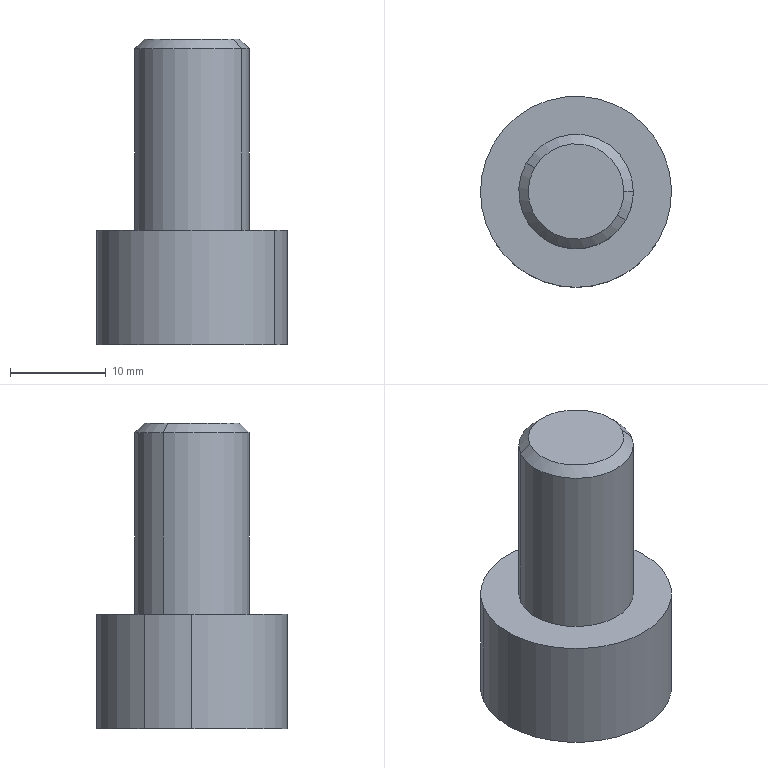Part | SolidWorks | features BaseBody 1 | 1 solid | 19 faces | box 20 x 20 x 32 mm | volume 5504 mm3 | plane 10 | cylinder 6 | cone 3 | commonest cylinder face diameters 12 x3 20 x3
STEP:
#1=CARTESIAN_POINT('',(364.67,895.749,656.107));
#2=VERTEX_POINT('',#1);
#3=CARTESIAN_POINT('',(363.804,896.249,655.107));
#4=VERTEX_POINT('',#3);
#5=CARTESIAN_POINT('',(364.67,895.749,656.107));
#6=DIRECTION('',(-0.6124,0.3536,-0.7071));
#7=VECTOR('',#6,1000.);
#8=LINE('',#5,#7);
#9=EDGE_CURVE('',#2,#4,#8,.T.);
#10=ORIENTED_EDGE('',*,*,#9,.T.);
#11=CARTESIAN_POINT('',(374.196,890.249,655.107));
#12=VERTEX_POINT('',#11);
#13=CARTESIAN_POINT('',(369.,893.249,655.107));
#14=DIRECTION('',(0.,0.,1.));
#15=DIRECTION('',(-0.866,0.5,0.));
#16=AXIS2_PLACEMENT_3D('',#13,#14,#15);
#17=CIRCLE('',#16,6.);
#18=EDGE_CURVE('',#4,#12,#17,.T.);
#19=ORIENTED_EDGE('',*,*,#18,.T.);
#20=CARTESIAN_POINT('',(373.33,890.749,656.107));
#21=VERTEX_POINT('',#20);
#22=CARTESIAN_POINT('',(373.33,890.749,656.107));
#23=DIRECTION('',(0.6124,-0.3536,-0.7071));
#24=VECTOR('',#23,1000.);
#25=LINE('',#22,#24);
#26=EDGE_CURVE('',#21,#12,#25,.T.);
#27=ORIENTED_EDGE('',*,*,#26,.F.);
#28=CARTESIAN_POINT('',(369.,893.249,656.107));
#29=DIRECTION('',(0.,0.,-1.));
#30=DIRECTION('',(-0.866,0.5,0.));
#31=AXIS2_PLACEMENT_3D('',#28,#29,#30);
#32=CIRCLE('',#31,5.);
#33=EDGE_CURVE('',#21,#2,#32,.T.);
#34=ORIENTED_EDGE('',*,*,#33,.T.);
#35=EDGE_LOOP('',(#10,#19,#27,#34));
#36=FACE_OUTER_BOUND('',#35,.T.);
#37=CARTESIAN_POINT('',(369.,893.249,656.107));
#38=DIRECTION('',(0.,0.,-1.));
#39=DIRECTION('',(1.,0.,0.));
#40=AXIS2_PLACEMENT_3D('',#37,#38,#39);
#41=CONICAL_SURFACE('',#40,5.,0.7854);
#42=ADVANCED_FACE('',(#36),#41,.T.);
#43=ORIENTED_EDGE('',*,*,#33,.F.);
#44=CARTESIAN_POINT('',(374.,893.249,656.107));
#45=VERTEX_POINT('',#44);
#46=CARTESIAN_POINT('',(369.,893.249,656.107));
#47=DIRECTION('',(0.,0.,-1.));
#48=DIRECTION('',(-0.866,0.5,0.));
#49=AXIS2_PLACEMENT_3D('',#46,#47,#48);
#50=CIRCLE('',#49,5.);
#51=EDGE_CURVE('',#45,#21,#50,.T.);
#52=ORIENTED_EDGE('',*,*,#51,.F.);
#53=CARTESIAN_POINT('',(369.,893.249,656.107));
#54=DIRECTION('',(0.,0.,-1.));
#55=DIRECTION('',(-0.866,0.5,0.));
#56=AXIS2_PLACEMENT_3D('',#53,#54,#55);
#57=CIRCLE('',#56,5.);
#58=EDGE_CURVE('',#2,#45,#57,.T.);
#59=ORIENTED_EDGE('',*,*,#58,.F.);
#60=EDGE_LOOP('',(#43,#52,#59));
#61=FACE_OUTER_BOUND('',#60,.T.);
#62=CARTESIAN_POINT('',(369.,893.249,656.107));
#63=DIRECTION('',(0.,0.,1.));
#64=DIRECTION('',(1.,0.,0.));
#65=AXIS2_PLACEMENT_3D('',#62,#63,#64);
#66=PLANE('',#65);
#67=ADVANCED_FACE('',(#61),#66,.T.);
#68=CARTESIAN_POINT('',(363.804,896.249,636.107));
#69=VERTEX_POINT('',#68);
#70=CARTESIAN_POINT('',(363.804,896.249,656.107));
#71=DIRECTION('',(0.,0.,-1.));
#72=VECTOR('',#71,1000.);
#73=LINE('',#70,#72);
#74=EDGE_CURVE('',#4,#69,#73,.T.);
#75=ORIENTED_EDGE('',*,*,#74,.T.);
#76=CARTESIAN_POINT('',(374.196,890.249,636.107));
#77=VERTEX_POINT('',#76);
#78=CARTESIAN_POINT('',(369.,893.249,636.107));
#79=DIRECTION('',(0.,0.,-1.));
#80=DIRECTION('',(0.866,-0.5,0.));
#81=AXIS2_PLACEMENT_3D('',#78,#79,#80);
#82=CIRCLE('',#81,6.);
#83=EDGE_CURVE('',#77,#69,#82,.T.);
#84=ORIENTED_EDGE('',*,*,#83,.F.);
#85=CARTESIAN_POINT('',(374.196,890.249,656.107));
#86=DIRECTION('',(0.,0.,-1.));
#87=VECTOR('',#86,1000.);
#88=LINE('',#85,#87);
#89=EDGE_CURVE('',#12,#77,#88,.T.);
#90=ORIENTED_EDGE('',*,*,#89,.F.);
#91=ORIENTED_EDGE('',*,*,#18,.F.);
#92=EDGE_LOOP('',(#75,#84,#90,#91));
#93=FACE_OUTER_BOUND('',#92,.T.);
#94=CARTESIAN_POINT('',(369.,893.249,656.107));
#95=DIRECTION('',(0.,0.,-1.));
#96=DIRECTION('',(1.,0.,0.));
#97=AXIS2_PLACEMENT_3D('',#94,#95,#96);
#98=CYLINDRICAL_SURFACE('',#97,6.);
#99=ADVANCED_FACE('',(#93),#98,.T.);
#100=CARTESIAN_POINT('',(365.188,888.984,630.107));
#101=VERTEX_POINT('',#100);
#102=CARTESIAN_POINT('',(370.787,887.815,630.107));
#103=VERTEX_POINT('',#102);
#104=CARTESIAN_POINT('',(365.188,888.984,630.107));
#105=DIRECTION('',(0.9789,-0.2044,0.));
#106=VECTOR('',#105,1000.);
#107=LINE('',#104,#106);
#108=EDGE_CURVE('',#101,#103,#107,.T.);
#109=ORIENTED_EDGE('',*,*,#108,.F.);
#110=CARTESIAN_POINT('',(363.401,894.418,630.107));
#111=VERTEX_POINT('',#110);
#112=CARTESIAN_POINT('',(363.401,894.418,630.107));
#113=DIRECTION('',(0.3124,-0.9499,0.));
#114=VECTOR('',#113,1000.);
#115=LINE('',#112,#114);
#116=EDGE_CURVE('',#111,#101,#115,.T.);
#117=ORIENTED_EDGE('',*,*,#116,.F.);
#118=CARTESIAN_POINT('',(367.213,898.683,630.107));
#119=VERTEX_POINT('',#118);
#120=CARTESIAN_POINT('',(367.213,898.683,630.107));
#121=DIRECTION('',(-0.6665,-0.7455,0.));
#122=VECTOR('',#121,1000.);
#123=LINE('',#120,#122);
#124=EDGE_CURVE('',#119,#111,#123,.T.);
#125=ORIENTED_EDGE('',*,*,#124,.F.);
#126=CARTESIAN_POINT('',(372.812,897.513,630.107));
#127=VERTEX_POINT('',#126);
#128=CARTESIAN_POINT('',(372.812,897.513,630.107));
#129=DIRECTION('',(-0.9789,0.2044,0.));
#130=VECTOR('',#129,1000.);
#131=LINE('',#128,#130);
#132=EDGE_CURVE('',#127,#119,#131,.T.);
#133=ORIENTED_EDGE('',*,*,#132,.F.);
#134=CARTESIAN_POINT('',(374.599,892.08,630.107));
#135=VERTEX_POINT('',#134);
#136=CARTESIAN_POINT('',(374.599,892.08,630.107));
#137=DIRECTION('',(-0.3124,0.9499,0.));
#138=VECTOR('',#137,1000.);
#139=LINE('',#136,#138);
#140=EDGE_CURVE('',#135,#127,#139,.T.);
#141=ORIENTED_EDGE('',*,*,#140,.F.);
#142=CARTESIAN_POINT('',(370.787,887.815,630.107));
#143=DIRECTION('',(0.6665,0.7455,0.));
#144=VECTOR('',#143,1000.);
#145=LINE('',#142,#144);
#146=EDGE_CURVE('',#103,#135,#145,.T.);
#147=ORIENTED_EDGE('',*,*,#146,.F.);
#148=EDGE_LOOP('',(#109,#117,#125,#133,#141,#147));
#149=FACE_OUTER_BOUND('',#148,.T.);
#150=CARTESIAN_POINT('',(370.787,887.815,630.107));
#151=DIRECTION('',(0.,0.,-1.));
#152=DIRECTION('',(0.,-1.,0.));
#153=AXIS2_PLACEMENT_3D('',#150,#151,#152);
#154=PLANE('',#153);
#155=ADVANCED_FACE('',(#149),#154,.T.);
#156=CARTESIAN_POINT('',(370.787,887.815,624.107));
#157=VERTEX_POINT('',#156);
#158=CARTESIAN_POINT('',(374.599,892.08,624.107));
#159=VERTEX_POINT('',#158);
#160=CARTESIAN_POINT('',(370.787,887.815,624.107));
#161=DIRECTION('',(0.6665,0.7455,0.));
#162=VECTOR('',#161,1000.);
#163=LINE('',#160,#162);
#164=EDGE_CURVE('',#157,#159,#163,.T.);
#165=ORIENTED_EDGE('',*,*,#164,.F.);
#166=CARTESIAN_POINT('',(370.787,887.815,630.107));
#167=DIRECTION('',(0.,0.,-1.));
#168=VECTOR('',#167,1000.);
#169=LINE('',#166,#168);
#170=EDGE_CURVE('',#103,#157,#169,.T.);
#171=ORIENTED_EDGE('',*,*,#170,.F.);
#172=ORIENTED_EDGE('',*,*,#146,.T.);
#173=CARTESIAN_POINT('',(374.599,892.08,630.107));
#174=DIRECTION('',(0.,0.,-1.));
#175=VECTOR('',#174,1000.);
#176=LINE('',#173,#175);
#177=EDGE_CURVE('',#135,#159,#176,.T.);
#178=ORIENTED_EDGE('',*,*,#177,.T.);
#179=EDGE_LOOP('',(#165,#171,#172,#178));
#180=FACE_OUTER_BOUND('',#179,.T.);
#181=CARTESIAN_POINT('',(370.787,887.815,630.107));
#182=DIRECTION('',(0.7455,-0.6665,0.));
#183=DIRECTION('',(0.,0.,-1.));
#184=AXIS2_PLACEMENT_3D('',#181,#182,#183);
#185=PLANE('',#184);
#186=ADVANCED_FACE('',(#180),#185,.F.);
#187=CARTESIAN_POINT('',(372.812,897.513,624.107));
#188=VERTEX_POINT('',#187);
#189=CARTESIAN_POINT('',(374.599,892.08,624.107));
#190=DIRECTION('',(-0.3124,0.9499,0.));
#191=VECTOR('',#190,1000.);
#192=LINE('',#189,#191);
#193=EDGE_CURVE('',#159,#188,#192,.T.);
#194=ORIENTED_EDGE('',*,*,#193,.F.);
#195=ORIENTED_EDGE('',*,*,#177,.F.);
#196=ORIENTED_EDGE('',*,*,#140,.T.);
#197=CARTESIAN_POINT('',(372.812,897.513,630.107));
#198=DIRECTION('',(0.,0.,-1.));
#199=VECTOR('',#198,1000.);
#200=LINE('',#197,#199);
#201=EDGE_CURVE('',#127,#188,#200,.T.);
#202=ORIENTED_EDGE('',*,*,#201,.T.);
#203=EDGE_LOOP('',(#194,#195,#196,#202));
#204=FACE_OUTER_BOUND('',#203,.T.);
#205=CARTESIAN_POINT('',(374.599,892.08,630.107));
#206=DIRECTION('',(0.9499,0.3124,0.));
#207=DIRECTION('',(0.,0.,-1.));
#208=AXIS2_PLACEMENT_3D('',#205,#206,#207);
#209=PLANE('',#208);
#210=ADVANCED_FACE('',(#204),#209,.F.);
#211=CARTESIAN_POINT('',(367.213,898.683,624.107));
#212=VERTEX_POINT('',#211);
#213=CARTESIAN_POINT('',(372.812,897.513,624.107));
#214=DIRECTION('',(-0.9789,0.2044,0.));
#215=VECTOR('',#214,1000.);
#216=LINE('',#213,#215);
#217=EDGE_CURVE('',#188,#212,#216,.T.);
#218=ORIENTED_EDGE('',*,*,#217,.F.);
#219=ORIENTED_EDGE('',*,*,#201,.F.);
#220=ORIENTED_EDGE('',*,*,#132,.T.);
#221=CARTESIAN_POINT('',(367.213,898.683,630.107));
#222=DIRECTION('',(0.,0.,-1.));
#223=VECTOR('',#222,1000.);
#224=LINE('',#221,#223);
#225=EDGE_CURVE('',#119,#212,#224,.T.);
#226=ORIENTED_EDGE('',*,*,#225,.T.);
#227=EDGE_LOOP('',(#218,#219,#220,#226));
#228=FACE_OUTER_BOUND('',#227,.T.);
#229=CARTESIAN_POINT('',(372.812,897.513,630.107));
#230=DIRECTION('',(0.2044,0.9789,0.));
#231=DIRECTION('',(0.,0.,-1.));
#232=AXIS2_PLACEMENT_3D('',#229,#230,#231);
#233=PLANE('',#232);
#234=ADVANCED_FACE('',(#228),#233,.F.);
#235=CARTESIAN_POINT('',(363.401,894.418,624.107));
#236=VERTEX_POINT('',#235);
#237=CARTESIAN_POINT('',(367.213,898.683,624.107));
#238=DIRECTION('',(-0.6665,-0.7455,0.));
#239=VECTOR('',#238,1000.);
#240=LINE('',#237,#239);
#241=EDGE_CURVE('',#212,#236,#240,.T.);
#242=ORIENTED_EDGE('',*,*,#241,.F.);
#243=ORIENTED_EDGE('',*,*,#225,.F.);
#244=ORIENTED_EDGE('',*,*,#124,.T.);
#245=CARTESIAN_POINT('',(363.401,894.418,630.107));
#246=DIRECTION('',(0.,0.,-1.));
#247=VECTOR('',#246,1000.);
#248=LINE('',#245,#247);
#249=EDGE_CURVE('',#111,#236,#248,.T.);
#250=ORIENTED_EDGE('',*,*,#249,.T.);
#251=EDGE_LOOP('',(#242,#243,#244,#250));
#252=FACE_OUTER_BOUND('',#251,.T.);
#253=CARTESIAN_POINT('',(367.213,898.683,630.107));
#254=DIRECTION('',(-0.7455,0.6665,0.));
#255=DIRECTION('',(0.,0.,1.));
#256=AXIS2_PLACEMENT_3D('',#253,#254,#255);
#257=PLANE('',#256);
#258=ADVANCED_FACE('',(#252),#257,.F.);
#259=CARTESIAN_POINT('',(365.188,888.984,624.107));
#260=VERTEX_POINT('',#259);
#261=CARTESIAN_POINT('',(363.401,894.418,624.107));
#262=DIRECTION('',(0.3124,-0.9499,0.));
#263=VECTOR('',#262,1000.);
#264=LINE('',#261,#263);
#265=EDGE_CURVE('',#236,#260,#264,.T.);
#266=ORIENTED_EDGE('',*,*,#265,.F.);
#267=ORIENTED_EDGE('',*,*,#249,.F.);
#268=ORIENTED_EDGE('',*,*,#116,.T.);
#269=CARTESIAN_POINT('',(365.188,888.984,630.107));
#270=DIRECTION('',(0.,0.,-1.));
#271=VECTOR('',#270,1000.);
#272=LINE('',#269,#271);
#273=EDGE_CURVE('',#101,#260,#272,.T.);
#274=ORIENTED_EDGE('',*,*,#273,.T.);
#275=EDGE_LOOP('',(#266,#267,#268,#274));
#276=FACE_OUTER_BOUND('',#275,.T.);
#277=CARTESIAN_POINT('',(363.401,894.418,630.107));
#278=DIRECTION('',(-0.9499,-0.3124,0.));
#279=DIRECTION('',(-0.3124,0.9499,0.));
#280=AXIS2_PLACEMENT_3D('',#277,#278,#279);
#281=PLANE('',#280);
#282=ADVANCED_FACE('',(#276),#281,.F.);
#283=CARTESIAN_POINT('',(365.188,888.984,624.107));
#284=DIRECTION('',(0.9789,-0.2044,0.));
#285=VECTOR('',#284,1000.);
#286=LINE('',#283,#285);
#287=EDGE_CURVE('',#260,#157,#286,.T.);
#288=ORIENTED_EDGE('',*,*,#287,.F.);
#289=ORIENTED_EDGE('',*,*,#273,.F.);
#290=ORIENTED_EDGE('',*,*,#108,.T.);
#291=ORIENTED_EDGE('',*,*,#170,.T.);
#292=EDGE_LOOP('',(#288,#289,#290,#291));
#293=FACE_OUTER_BOUND('',#292,.T.);
#294=CARTESIAN_POINT('',(365.188,888.984,630.107));
#295=DIRECTION('',(-0.2044,-0.9789,0.));
#296=DIRECTION('',(-0.9789,0.2044,0.));
#297=AXIS2_PLACEMENT_3D('',#294,#295,#296);
#298=PLANE('',#297);
#299=ADVANCED_FACE('',(#293),#298,.F.);
#300=ORIENTED_EDGE('',*,*,#287,.T.);
#301=ORIENTED_EDGE('',*,*,#164,.T.);
#302=ORIENTED_EDGE('',*,*,#193,.T.);
#303=ORIENTED_EDGE('',*,*,#217,.T.);
#304=ORIENTED_EDGE('',*,*,#241,.T.);
#305=ORIENTED_EDGE('',*,*,#265,.T.);
#306=EDGE_LOOP('',(#300,#301,#302,#303,#304,#305));
#307=FACE_BOUND('',#306,.T.);
#308=CARTESIAN_POINT('',(360.34,898.249,624.107));
#309=VERTEX_POINT('',#308);
#310=CARTESIAN_POINT('',(359.,893.249,624.107));
#311=VERTEX_POINT('',#310);
#312=CARTESIAN_POINT('',(369.,893.249,624.107));
#313=DIRECTION('',(0.,0.,1.));
#314=DIRECTION('',(0.866,-0.5,0.));
#315=AXIS2_PLACEMENT_3D('',#312,#313,#314);
#316=CIRCLE('',#315,10.);
#317=EDGE_CURVE('',#309,#311,#316,.T.);
#318=ORIENTED_EDGE('',*,*,#317,.F.);
#319=CARTESIAN_POINT('',(377.66,888.249,624.107));
#320=VERTEX_POINT('',#319);
#321=CARTESIAN_POINT('',(369.,893.249,624.107));
#322=DIRECTION('',(0.,0.,1.));
#323=DIRECTION('',(0.866,-0.5,0.));
#324=AXIS2_PLACEMENT_3D('',#321,#322,#323);
#325=CIRCLE('',#324,10.);
#326=EDGE_CURVE('',#320,#309,#325,.T.);
#327=ORIENTED_EDGE('',*,*,#326,.F.);
#328=CARTESIAN_POINT('',(369.,893.249,624.107));
#329=DIRECTION('',(0.,0.,1.));
#330=DIRECTION('',(0.866,-0.5,0.));
#331=AXIS2_PLACEMENT_3D('',#328,#329,#330);
#332=CIRCLE('',#331,10.);
#333=EDGE_CURVE('',#311,#320,#332,.T.);
#334=ORIENTED_EDGE('',*,*,#333,.F.);
#335=EDGE_LOOP('',(#318,#327,#334));
#336=FACE_OUTER_BOUND('',#335,.T.);
#337=CARTESIAN_POINT('',(369.,893.249,624.107));
#338=DIRECTION('',(0.,0.,-1.));
#339=DIRECTION('',(0.,-1.,0.));
#340=AXIS2_PLACEMENT_3D('',#337,#338,#339);
#341=PLANE('',#340);
#342=ADVANCED_FACE('',(#307,#336),#341,.T.);
#343=CARTESIAN_POINT('',(359.,893.249,636.107));
#344=VERTEX_POINT('',#343);
#345=CARTESIAN_POINT('',(359.,893.249,624.107));
#346=DIRECTION('',(0.,0.,1.));
#347=VECTOR('',#346,1000.);
#348=LINE('',#345,#347);
#349=EDGE_CURVE('',#311,#344,#348,.T.);
#350=ORIENTED_EDGE('',*,*,#349,.F.);
#351=ORIENTED_EDGE('',*,*,#333,.T.);
#352=CARTESIAN_POINT('',(377.66,888.249,636.107));
#353=VERTEX_POINT('',#352);
#354=CARTESIAN_POINT('',(377.66,888.249,624.107));
#355=DIRECTION('',(0.,0.,1.));
#356=VECTOR('',#355,1000.);
#357=LINE('',#354,#356);
#358=EDGE_CURVE('',#320,#353,#357,.T.);
#359=ORIENTED_EDGE('',*,*,#358,.T.);
#360=CARTESIAN_POINT('',(369.,893.249,636.107));
#361=DIRECTION('',(0.,0.,1.));
#362=DIRECTION('',(0.866,-0.5,0.));
#363=AXIS2_PLACEMENT_3D('',#360,#361,#362);
#364=CIRCLE('',#363,10.);
#365=EDGE_CURVE('',#344,#353,#364,.T.);
#366=ORIENTED_EDGE('',*,*,#365,.F.);
#367=EDGE_LOOP('',(#350,#351,#359,#366));
#368=FACE_OUTER_BOUND('',#367,.T.);
#369=CARTESIAN_POINT('',(369.,893.249,624.107));
#370=DIRECTION('',(0.,0.,1.));
#371=DIRECTION('',(-1.,0.,0.));
#372=AXIS2_PLACEMENT_3D('',#369,#370,#371);
#373=CYLINDRICAL_SURFACE('',#372,10.);
#374=ADVANCED_FACE('',(#368),#373,.T.);
#375=ORIENTED_EDGE('',*,*,#83,.T.);
#376=CARTESIAN_POINT('',(375.,893.249,636.107));
#377=VERTEX_POINT('',#376);
#378=CARTESIAN_POINT('',(369.,893.249,636.107));
#379=DIRECTION('',(0.,0.,-1.));
#380=DIRECTION('',(0.866,-0.5,0.));
#381=AXIS2_PLACEMENT_3D('',#378,#379,#380);
#382=CIRCLE('',#381,6.);
#383=EDGE_CURVE('',#69,#377,#382,.T.);
#384=ORIENTED_EDGE('',*,*,#383,.T.);
#385=CARTESIAN_POINT('',(369.,893.249,636.107));
#386=DIRECTION('',(0.,0.,-1.));
#387=DIRECTION('',(0.866,-0.5,0.));
#388=AXIS2_PLACEMENT_3D('',#385,#386,#387);
#389=CIRCLE('',#388,6.);
#390=EDGE_CURVE('',#377,#77,#389,.T.);
#391=ORIENTED_EDGE('',*,*,#390,.T.);
#392=EDGE_LOOP('',(#375,#384,#391));
#393=FACE_BOUND('',#392,.T.);
#394=CARTESIAN_POINT('',(360.34,898.249,636.107));
#395=VERTEX_POINT('',#394);
#396=CARTESIAN_POINT('',(369.,893.249,636.107));
#397=DIRECTION('',(0.,0.,1.));
#398=DIRECTION('',(0.866,-0.5,0.));
#399=AXIS2_PLACEMENT_3D('',#396,#397,#398);
#400=CIRCLE('',#399,10.);
#401=EDGE_CURVE('',#395,#344,#400,.T.);
#402=ORIENTED_EDGE('',*,*,#401,.T.);
#403=ORIENTED_EDGE('',*,*,#365,.T.);
#404=CARTESIAN_POINT('',(369.,893.249,636.107));
#405=DIRECTION('',(0.,0.,1.));
#406=DIRECTION('',(0.866,-0.5,0.));
#407=AXIS2_PLACEMENT_3D('',#404,#405,#406);
#408=CIRCLE('',#407,10.);
#409=EDGE_CURVE('',#353,#395,#408,.T.);
#410=ORIENTED_EDGE('',*,*,#409,.T.);
#411=EDGE_LOOP('',(#402,#403,#410));
#412=FACE_OUTER_BOUND('',#411,.T.);
#413=CARTESIAN_POINT('',(369.,893.249,636.107));
#414=DIRECTION('',(0.,0.,-1.));
#415=DIRECTION('',(0.,-1.,0.));
#416=AXIS2_PLACEMENT_3D('',#413,#414,#415);
#417=PLANE('',#416);
#418=ADVANCED_FACE('',(#393,#412),#417,.F.);
#419=ORIENTED_EDGE('',*,*,#326,.T.);
#420=CARTESIAN_POINT('',(360.34,898.249,624.107));
#421=DIRECTION('',(0.,0.,1.));
#422=VECTOR('',#421,1000.);
#423=LINE('',#420,#422);
#424=EDGE_CURVE('',#309,#395,#423,.T.);
#425=ORIENTED_EDGE('',*,*,#424,.T.);
#426=ORIENTED_EDGE('',*,*,#409,.F.);
#427=ORIENTED_EDGE('',*,*,#358,.F.);
#428=EDGE_LOOP('',(#419,#425,#426,#427));
#429=FACE_OUTER_BOUND('',#428,.T.);
#430=CARTESIAN_POINT('',(369.,893.249,624.107));
#431=DIRECTION('',(0.,0.,1.));
#432=DIRECTION('',(-1.,0.,0.));
#433=AXIS2_PLACEMENT_3D('',#430,#431,#432);
#434=CYLINDRICAL_SURFACE('',#433,10.);
#435=ADVANCED_FACE('',(#429),#434,.T.);
#436=CARTESIAN_POINT('',(375.,893.249,655.107));
#437=VERTEX_POINT('',#436);
#438=CARTESIAN_POINT('',(375.,893.249,656.107));
#439=DIRECTION('',(0.,0.,-1.));
#440=VECTOR('',#439,1000.);
#441=LINE('',#438,#440);
#442=EDGE_CURVE('',#437,#377,#441,.T.);
#443=ORIENTED_EDGE('',*,*,#442,.F.);
#444=CARTESIAN_POINT('',(369.,893.249,655.107));
#445=DIRECTION('',(0.,0.,1.));
#446=DIRECTION('',(-0.866,0.5,0.));
#447=AXIS2_PLACEMENT_3D('',#444,#445,#446);
#448=CIRCLE('',#447,6.);
#449=EDGE_CURVE('',#12,#437,#448,.T.);
#450=ORIENTED_EDGE('',*,*,#449,.F.);
#451=ORIENTED_EDGE('',*,*,#89,.T.);
#452=ORIENTED_EDGE('',*,*,#390,.F.);
#453=EDGE_LOOP('',(#443,#450,#451,#452));
#454=FACE_OUTER_BOUND('',#453,.T.);
#455=CARTESIAN_POINT('',(369.,893.249,656.107));
#456=DIRECTION('',(0.,0.,-1.));
#457=DIRECTION('',(1.,0.,0.));
#458=AXIS2_PLACEMENT_3D('',#455,#456,#457);
#459=CYLINDRICAL_SURFACE('',#458,6.);
#460=ADVANCED_FACE('',(#454),#459,.T.);
#461=CARTESIAN_POINT('',(374.,893.249,656.107));
#462=DIRECTION('',(0.7071,0.,-0.7071));
#463=VECTOR('',#462,1000.);
#464=LINE('',#461,#463);
#465=EDGE_CURVE('',#45,#437,#464,.T.);
#466=ORIENTED_EDGE('',*,*,#465,.F.);
#467=ORIENTED_EDGE('',*,*,#51,.T.);
#468=ORIENTED_EDGE('',*,*,#26,.T.);
#469=ORIENTED_EDGE('',*,*,#449,.T.);
#470=EDGE_LOOP('',(#466,#467,#468,#469));
#471=FACE_OUTER_BOUND('',#470,.T.);
#472=CARTESIAN_POINT('',(369.,893.249,656.107));
#473=DIRECTION('',(0.,0.,-1.));
#474=DIRECTION('',(1.,0.,0.));
#475=AXIS2_PLACEMENT_3D('',#472,#473,#474);
#476=CONICAL_SURFACE('',#475,5.,0.7854);
#477=ADVANCED_FACE('',(#471),#476,.T.);
#478=ORIENTED_EDGE('',*,*,#58,.T.);
#479=ORIENTED_EDGE('',*,*,#465,.T.);
#480=CARTESIAN_POINT('',(369.,893.249,655.107));
#481=DIRECTION('',(0.,0.,1.));
#482=DIRECTION('',(-0.866,0.5,0.));
#483=AXIS2_PLACEMENT_3D('',#480,#481,#482);
#484=CIRCLE('',#483,6.);
#485=EDGE_CURVE('',#437,#4,#484,.T.);
#486=ORIENTED_EDGE('',*,*,#485,.T.);
#487=ORIENTED_EDGE('',*,*,#9,.F.);
#488=EDGE_LOOP('',(#478,#479,#486,#487));
#489=FACE_OUTER_BOUND('',#488,.T.);
#490=CARTESIAN_POINT('',(369.,893.249,656.107));
#491=DIRECTION('',(0.,0.,-1.));
#492=DIRECTION('',(1.,0.,0.));
#493=AXIS2_PLACEMENT_3D('',#490,#491,#492);
#494=CONICAL_SURFACE('',#493,5.,0.7854);
#495=ADVANCED_FACE('',(#489),#494,.T.);
#496=ORIENTED_EDGE('',*,*,#485,.F.);
#497=ORIENTED_EDGE('',*,*,#442,.T.);
#498=ORIENTED_EDGE('',*,*,#383,.F.);
#499=ORIENTED_EDGE('',*,*,#74,.F.);
#500=EDGE_LOOP('',(#496,#497,#498,#499));
#501=FACE_OUTER_BOUND('',#500,.T.);
#502=CARTESIAN_POINT('',(369.,893.249,656.107));
#503=DIRECTION('',(0.,0.,-1.));
#504=DIRECTION('',(1.,0.,0.));
#505=AXIS2_PLACEMENT_3D('',#502,#503,#504);
#506=CYLINDRICAL_SURFACE('',#505,6.);
#507=ADVANCED_FACE('',(#501),#506,.T.);
#508=ORIENTED_EDGE('',*,*,#317,.T.);
#509=ORIENTED_EDGE('',*,*,#349,.T.);
#510=ORIENTED_EDGE('',*,*,#401,.F.);
#511=ORIENTED_EDGE('',*,*,#424,.F.);
#512=EDGE_LOOP('',(#508,#509,#510,#511));
#513=FACE_OUTER_BOUND('',#512,.T.);
#514=CARTESIAN_POINT('',(369.,893.249,624.107));
#515=DIRECTION('',(0.,0.,1.));
#516=DIRECTION('',(-1.,0.,0.));
#517=AXIS2_PLACEMENT_3D('',#514,#515,#516);
#518=CYLINDRICAL_SURFACE('',#517,10.);
#519=ADVANCED_FACE('',(#513),#518,.T.);
#520=CLOSED_SHELL('',(#42,#67,#99,#155,#186,#210,#234,#258,#282,#299,#342,#374,#418,#435,#460,#477,#495,#507,#519));
#521=MANIFOLD_SOLID_BREP('',#520);
#522=CARTESIAN_POINT('',(0.,0.,0.));
#523=DIRECTION('',(0.,0.,1.));
#524=DIRECTION('',(1.,0.,0.));
#525=AXIS2_PLACEMENT_3D('',#522,#523,#524);
#526=(LENGTH_UNIT()NAMED_UNIT(*)SI_UNIT(.MILLI.,.METRE.));
#527=UNCERTAINTY_MEASURE_WITH_UNIT(LENGTH_MEASURE(0.00001),#526,'','');
#528=(NAMED_UNIT(*)PLANE_ANGLE_UNIT()SI_UNIT($,.RADIAN.));
#529=(NAMED_UNIT(*)SI_UNIT($,.STERADIAN.)SOLID_ANGLE_UNIT());
#530=(GEOMETRIC_REPRESENTATION_CONTEXT(3)GLOBAL_UNCERTAINTY_ASSIGNED_CONTEXT((#527))GLOBAL_UNIT_ASSIGNED_CONTEXT((#526,#528,#529))REPRESENTATION_CONTEXT('',''));
#531=ADVANCED_BREP_SHAPE_REPRESENTATION('',(#521,#525),#530);